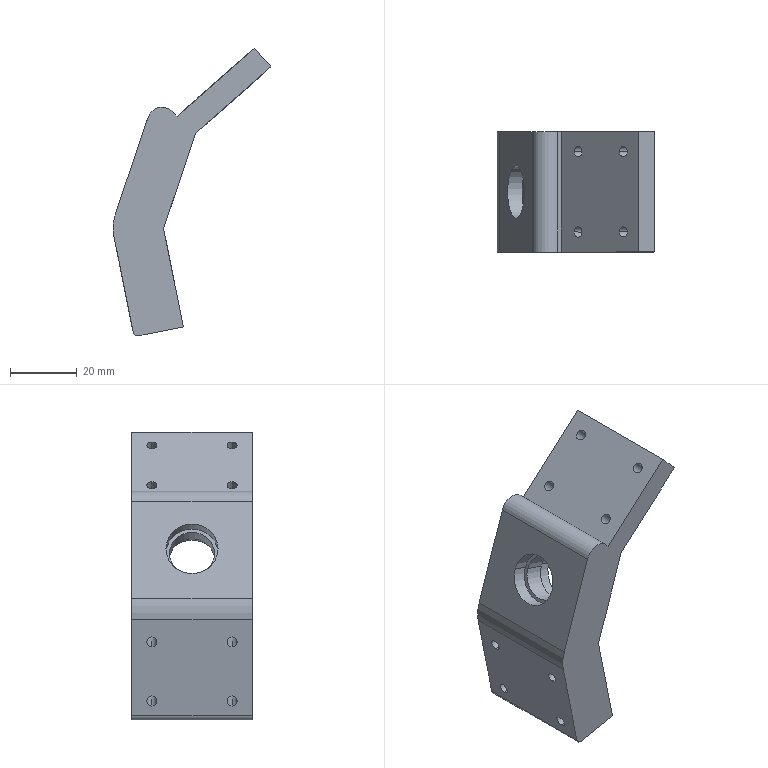Part | STEP file | 2026.6.15-Main Assembly图.sldasm-Part-275 | 1 solid | 38 faces | box 47.222 x 36 x 85.968 mm | volume 40942 mm3 | cylinder 25 | plane 13 | commonest cylinder face diameters 3.06 x16 15.6 x4 13.5 x2 3 x1 9 x1 24 x1
STEP:
#1=CARTESIAN_POINT('',(-1656.869,1431.014,3245.304));
#2=VERTEX_POINT('',#1);
#3=CARTESIAN_POINT('',(-1662.554,1431.014,3247.224));
#4=VERTEX_POINT('',#3);
#5=CARTESIAN_POINT('',(-1638.394,1431.014,3239.065));
#6=DIRECTION('',(-0.9474,0.,0.3199));
#7=VECTOR('',#6,1000.);
#8=LINE('',#5,#7);
#9=EDGE_CURVE('',#2,#4,#8,.T.);
#10=ORIENTED_EDGE('',*,*,#9,.F.);
#11=CARTESIAN_POINT('',(-1656.869,1417.514,3245.304));
#12=VERTEX_POINT('',#11);
#13=CARTESIAN_POINT('',(-1656.869,1424.264,3245.304));
#14=DIRECTION('',(-0.9474,0.,0.3199));
#15=DIRECTION('',(0.,-1.,0.));
#16=AXIS2_PLACEMENT_3D('',#13,#14,#15);
#17=CIRCLE('',#16,6.75);
#18=EDGE_CURVE('',#12,#2,#17,.T.);
#19=ORIENTED_EDGE('',*,*,#18,.F.);
#20=CARTESIAN_POINT('',(-1662.554,1417.514,3247.224));
#21=VERTEX_POINT('',#20);
#22=CARTESIAN_POINT('',(-1638.394,1417.514,3239.065));
#23=DIRECTION('',(-0.9474,0.,0.3199));
#24=VECTOR('',#23,1000.);
#25=LINE('',#22,#24);
#26=EDGE_CURVE('',#12,#21,#25,.T.);
#27=ORIENTED_EDGE('',*,*,#26,.T.);
#28=CARTESIAN_POINT('',(-1662.554,1424.264,3247.224));
#29=DIRECTION('',(0.9474,0.,-0.3199));
#30=DIRECTION('',(0.,-1.,0.));
#31=AXIS2_PLACEMENT_3D('',#28,#29,#30);
#32=CIRCLE('',#31,6.75);
#33=EDGE_CURVE('',#4,#21,#32,.T.);
#34=ORIENTED_EDGE('',*,*,#33,.F.);
#35=EDGE_LOOP('',(#10,#19,#27,#34));
#36=FACE_OUTER_BOUND('',#35,.T.);
#37=CARTESIAN_POINT('',(-1638.394,1424.264,3239.065));
#38=DIRECTION('',(-0.9474,0.,0.3199));
#39=DIRECTION('',(0.,1.,0.));
#40=AXIS2_PLACEMENT_3D('',#37,#38,#39);
#41=CYLINDRICAL_SURFACE('',#40,6.75);
#42=ADVANCED_FACE('',(#36),#41,.F.);
#43=CARTESIAN_POINT('',(-1662.554,1416.464,3247.224));
#44=VERTEX_POINT('',#43);
#45=CARTESIAN_POINT('',(-1662.554,1432.064,3247.224));
#46=VERTEX_POINT('',#45);
#47=CARTESIAN_POINT('',(-1662.554,1424.264,3247.224));
#48=DIRECTION('',(-0.9474,0.,0.3199));
#49=DIRECTION('',(0.,-1.,0.));
#50=AXIS2_PLACEMENT_3D('',#47,#48,#49);
#51=CIRCLE('',#50,7.8);
#52=EDGE_CURVE('',#44,#46,#51,.T.);
#53=ORIENTED_EDGE('',*,*,#52,.T.);
#54=CARTESIAN_POINT('',(-1662.554,1424.264,3247.224));
#55=DIRECTION('',(-0.9474,0.,0.3199));
#56=DIRECTION('',(0.,-1.,0.));
#57=AXIS2_PLACEMENT_3D('',#54,#55,#56);
#58=CIRCLE('',#57,7.8);
#59=EDGE_CURVE('',#46,#44,#58,.T.);
#60=ORIENTED_EDGE('',*,*,#59,.T.);
#61=EDGE_LOOP('',(#53,#60));
#62=FACE_OUTER_BOUND('',#61,.T.);
#63=CARTESIAN_POINT('',(-1662.554,1424.264,3247.224));
#64=DIRECTION('',(0.9474,0.,-0.3199));
#65=DIRECTION('',(0.,-1.,0.));
#66=AXIS2_PLACEMENT_3D('',#63,#64,#65);
#67=CIRCLE('',#66,6.75);
#68=EDGE_CURVE('',#21,#4,#67,.T.);
#69=ORIENTED_EDGE('',*,*,#68,.T.);
#70=ORIENTED_EDGE('',*,*,#33,.T.);
#71=EDGE_LOOP('',(#69,#70));
#72=FACE_BOUND('',#71,.T.);
#73=CARTESIAN_POINT('',(-1662.554,1424.264,3247.224));
#74=DIRECTION('',(-0.9474,0.,0.3199));
#75=DIRECTION('',(0.,1.,0.));
#76=AXIS2_PLACEMENT_3D('',#73,#74,#75);
#77=PLANE('',#76);
#78=ADVANCED_FACE('',(#62,#72),#77,.T.);
#79=CARTESIAN_POINT('',(-1656.869,1432.064,3245.304));
#80=VERTEX_POINT('',#79);
#81=CARTESIAN_POINT('',(-1656.869,1416.464,3245.304));
#82=VERTEX_POINT('',#81);
#83=CARTESIAN_POINT('',(-1656.869,1424.264,3245.304));
#84=DIRECTION('',(0.9474,0.,-0.3199));
#85=DIRECTION('',(0.,1.,0.));
#86=AXIS2_PLACEMENT_3D('',#83,#84,#85);
#87=CIRCLE('',#86,7.8);
#88=EDGE_CURVE('',#80,#82,#87,.T.);
#89=ORIENTED_EDGE('',*,*,#88,.T.);
#90=CARTESIAN_POINT('',(-1656.869,1424.264,3245.304));
#91=DIRECTION('',(0.9474,0.,-0.3199));
#92=DIRECTION('',(0.,1.,0.));
#93=AXIS2_PLACEMENT_3D('',#90,#91,#92);
#94=CIRCLE('',#93,7.8);
#95=EDGE_CURVE('',#82,#80,#94,.T.);
#96=ORIENTED_EDGE('',*,*,#95,.T.);
#97=EDGE_LOOP('',(#89,#96));
#98=FACE_OUTER_BOUND('',#97,.T.);
#99=ORIENTED_EDGE('',*,*,#18,.T.);
#100=CARTESIAN_POINT('',(-1656.869,1424.264,3245.304));
#101=DIRECTION('',(-0.9474,0.,0.3199));
#102=DIRECTION('',(0.,-1.,0.));
#103=AXIS2_PLACEMENT_3D('',#100,#101,#102);
#104=CIRCLE('',#103,6.75);
#105=EDGE_CURVE('',#2,#12,#104,.T.);
#106=ORIENTED_EDGE('',*,*,#105,.T.);
#107=EDGE_LOOP('',(#99,#106));
#108=FACE_BOUND('',#107,.T.);
#109=CARTESIAN_POINT('',(-1656.869,1424.264,3245.304));
#110=DIRECTION('',(0.9474,0.,-0.3199));
#111=DIRECTION('',(0.,-1.,0.));
#112=AXIS2_PLACEMENT_3D('',#109,#110,#111);
#113=PLANE('',#112);
#114=ADVANCED_FACE('',(#98,#108),#113,.T.);
#115=CARTESIAN_POINT('',(-1666.817,1432.064,3248.663));
#116=VERTEX_POINT('',#115);
#117=CARTESIAN_POINT('',(-1662.554,1432.064,3247.224));
#118=DIRECTION('',(-0.9474,0.,0.3199));
#119=VECTOR('',#118,1000.);
#120=LINE('',#117,#119);
#121=EDGE_CURVE('',#46,#116,#120,.T.);
#122=ORIENTED_EDGE('',*,*,#121,.F.);
#123=ORIENTED_EDGE('',*,*,#52,.F.);
#124=CARTESIAN_POINT('',(-1666.817,1416.464,3248.663));
#125=VERTEX_POINT('',#124);
#126=CARTESIAN_POINT('',(-1662.554,1416.464,3247.224));
#127=DIRECTION('',(-0.9474,0.,0.3199));
#128=VECTOR('',#127,1000.);
#129=LINE('',#126,#128);
#130=EDGE_CURVE('',#44,#125,#129,.T.);
#131=ORIENTED_EDGE('',*,*,#130,.T.);
#132=CARTESIAN_POINT('',(-1666.817,1424.264,3248.663));
#133=DIRECTION('',(-0.9474,0.,0.3199));
#134=DIRECTION('',(0.,-1.,0.));
#135=AXIS2_PLACEMENT_3D('',#132,#133,#134);
#136=CIRCLE('',#135,7.8);
#137=EDGE_CURVE('',#125,#116,#136,.T.);
#138=ORIENTED_EDGE('',*,*,#137,.T.);
#139=EDGE_LOOP('',(#122,#123,#131,#138));
#140=FACE_OUTER_BOUND('',#139,.T.);
#141=CARTESIAN_POINT('',(-1662.554,1424.264,3247.224));
#142=DIRECTION('',(-0.9474,0.,0.3199));
#143=DIRECTION('',(0.,1.,0.));
#144=AXIS2_PLACEMENT_3D('',#141,#142,#143);
#145=CYLINDRICAL_SURFACE('',#144,7.8);
#146=ADVANCED_FACE('',(#140),#145,.F.);
#147=CARTESIAN_POINT('',(-1655.924,1436.264,3222.27));
#148=VERTEX_POINT('',#147);
#149=CARTESIAN_POINT('',(-1670.631,1436.264,3219.32));
#150=VERTEX_POINT('',#149);
#151=CARTESIAN_POINT('',(-1655.924,1436.264,3222.27));
#152=DIRECTION('',(-0.9805,0.,-0.1966));
#153=VECTOR('',#152,1000.);
#154=LINE('',#151,#153);
#155=EDGE_CURVE('',#148,#150,#154,.T.);
#156=ORIENTED_EDGE('',*,*,#155,.T.);
#157=CARTESIAN_POINT('',(-1671.233,1436.264,3222.32));
#158=VERTEX_POINT('',#157);
#159=CARTESIAN_POINT('',(-1670.932,1436.264,3220.82));
#160=DIRECTION('',(-0.9805,0.,-0.1966));
#161=DIRECTION('',(-0.1966,0.,0.9805));
#162=AXIS2_PLACEMENT_3D('',#159,#160,#161);
#163=CIRCLE('',#162,1.53);
#164=EDGE_CURVE('',#150,#158,#163,.T.);
#165=ORIENTED_EDGE('',*,*,#164,.T.);
#166=CARTESIAN_POINT('',(-1656.526,1436.264,3225.27));
#167=VERTEX_POINT('',#166);
#168=CARTESIAN_POINT('',(-1656.526,1436.264,3225.27));
#169=DIRECTION('',(-0.9805,0.,-0.1966));
#170=VECTOR('',#169,1000.);
#171=LINE('',#168,#170);
#172=EDGE_CURVE('',#167,#158,#171,.T.);
#173=ORIENTED_EDGE('',*,*,#172,.F.);
#174=CARTESIAN_POINT('',(-1656.225,1436.264,3223.77));
#175=DIRECTION('',(0.9805,0.,0.1966));
#176=DIRECTION('',(-0.1966,0.,0.9805));
#177=AXIS2_PLACEMENT_3D('',#174,#175,#176);
#178=CIRCLE('',#177,1.53);
#179=EDGE_CURVE('',#167,#148,#178,.T.);
#180=ORIENTED_EDGE('',*,*,#179,.T.);
#181=EDGE_LOOP('',(#156,#165,#173,#180));
#182=FACE_OUTER_BOUND('',#181,.T.);
#183=CARTESIAN_POINT('',(-1656.225,1436.264,3223.77));
#184=DIRECTION('',(0.9805,0.,0.1966));
#185=DIRECTION('',(0.1966,0.,-0.9805));
#186=AXIS2_PLACEMENT_3D('',#183,#184,#185);
#187=CYLINDRICAL_SURFACE('',#186,1.53);
#188=ADVANCED_FACE('',(#182),#187,.F.);
#189=CARTESIAN_POINT('',(-1652.385,1436.264,3204.621));
#190=VERTEX_POINT('',#189);
#191=CARTESIAN_POINT('',(-1667.092,1436.264,3201.671));
#192=VERTEX_POINT('',#191);
#193=CARTESIAN_POINT('',(-1652.385,1436.264,3204.621));
#194=DIRECTION('',(-0.9805,0.,-0.1966));
#195=VECTOR('',#194,1000.);
#196=LINE('',#193,#195);
#197=EDGE_CURVE('',#190,#192,#196,.T.);
#198=ORIENTED_EDGE('',*,*,#197,.T.);
#199=CARTESIAN_POINT('',(-1667.694,1436.264,3204.672));
#200=VERTEX_POINT('',#199);
#201=CARTESIAN_POINT('',(-1667.393,1436.264,3203.172));
#202=DIRECTION('',(-0.9805,0.,-0.1966));
#203=DIRECTION('',(-0.1966,0.,0.9805));
#204=AXIS2_PLACEMENT_3D('',#201,#202,#203);
#205=CIRCLE('',#204,1.53);
#206=EDGE_CURVE('',#192,#200,#205,.T.);
#207=ORIENTED_EDGE('',*,*,#206,.T.);
#208=CARTESIAN_POINT('',(-1652.986,1436.264,3207.621));
#209=VERTEX_POINT('',#208);
#210=CARTESIAN_POINT('',(-1652.986,1436.264,3207.621));
#211=DIRECTION('',(-0.9805,0.,-0.1966));
#212=VECTOR('',#211,1000.);
#213=LINE('',#210,#212);
#214=EDGE_CURVE('',#209,#200,#213,.T.);
#215=ORIENTED_EDGE('',*,*,#214,.F.);
#216=CARTESIAN_POINT('',(-1652.686,1436.264,3206.121));
#217=DIRECTION('',(0.9805,0.,0.1966));
#218=DIRECTION('',(-0.1966,0.,0.9805));
#219=AXIS2_PLACEMENT_3D('',#216,#217,#218);
#220=CIRCLE('',#219,1.53);
#221=EDGE_CURVE('',#209,#190,#220,.T.);
#222=ORIENTED_EDGE('',*,*,#221,.T.);
#223=EDGE_LOOP('',(#198,#207,#215,#222));
#224=FACE_OUTER_BOUND('',#223,.T.);
#225=CARTESIAN_POINT('',(-1652.686,1436.264,3206.121));
#226=DIRECTION('',(0.9805,0.,0.1966));
#227=DIRECTION('',(0.1966,0.,-0.9805));
#228=AXIS2_PLACEMENT_3D('',#225,#226,#227);
#229=CYLINDRICAL_SURFACE('',#228,1.53);
#230=ADVANCED_FACE('',(#224),#229,.F.);
#231=CARTESIAN_POINT('',(-1655.924,1412.264,3222.27));
#232=VERTEX_POINT('',#231);
#233=CARTESIAN_POINT('',(-1670.631,1412.264,3219.32));
#234=VERTEX_POINT('',#233);
#235=CARTESIAN_POINT('',(-1655.924,1412.264,3222.27));
#236=DIRECTION('',(-0.9805,0.,-0.1966));
#237=VECTOR('',#236,1000.);
#238=LINE('',#235,#237);
#239=EDGE_CURVE('',#232,#234,#238,.T.);
#240=ORIENTED_EDGE('',*,*,#239,.T.);
#241=CARTESIAN_POINT('',(-1671.233,1412.264,3222.32));
#242=VERTEX_POINT('',#241);
#243=CARTESIAN_POINT('',(-1670.932,1412.264,3220.82));
#244=DIRECTION('',(-0.9805,0.,-0.1966));
#245=DIRECTION('',(-0.1966,0.,0.9805));
#246=AXIS2_PLACEMENT_3D('',#243,#244,#245);
#247=CIRCLE('',#246,1.53);
#248=EDGE_CURVE('',#234,#242,#247,.T.);
#249=ORIENTED_EDGE('',*,*,#248,.T.);
#250=CARTESIAN_POINT('',(-1656.526,1412.264,3225.27));
#251=VERTEX_POINT('',#250);
#252=CARTESIAN_POINT('',(-1656.526,1412.264,3225.27));
#253=DIRECTION('',(-0.9805,0.,-0.1966));
#254=VECTOR('',#253,1000.);
#255=LINE('',#252,#254);
#256=EDGE_CURVE('',#251,#242,#255,.T.);
#257=ORIENTED_EDGE('',*,*,#256,.F.);
#258=CARTESIAN_POINT('',(-1656.225,1412.264,3223.77));
#259=DIRECTION('',(0.9805,0.,0.1966));
#260=DIRECTION('',(-0.1966,0.,0.9805));
#261=AXIS2_PLACEMENT_3D('',#258,#259,#260);
#262=CIRCLE('',#261,1.53);
#263=EDGE_CURVE('',#251,#232,#262,.T.);
#264=ORIENTED_EDGE('',*,*,#263,.T.);
#265=EDGE_LOOP('',(#240,#249,#257,#264));
#266=FACE_OUTER_BOUND('',#265,.T.);
#267=CARTESIAN_POINT('',(-1656.225,1412.264,3223.77));
#268=DIRECTION('',(0.9805,0.,0.1966));
#269=DIRECTION('',(0.1966,0.,-0.9805));
#270=AXIS2_PLACEMENT_3D('',#267,#268,#269);
#271=CYLINDRICAL_SURFACE('',#270,1.53);
#272=ADVANCED_FACE('',(#266),#271,.F.);
#273=CARTESIAN_POINT('',(-1652.385,1412.264,3204.621));
#274=VERTEX_POINT('',#273);
#275=CARTESIAN_POINT('',(-1667.092,1412.264,3201.671));
#276=VERTEX_POINT('',#275);
#277=CARTESIAN_POINT('',(-1652.385,1412.264,3204.621));
#278=DIRECTION('',(-0.9805,0.,-0.1966));
#279=VECTOR('',#278,1000.);
#280=LINE('',#277,#279);
#281=EDGE_CURVE('',#274,#276,#280,.T.);
#282=ORIENTED_EDGE('',*,*,#281,.T.);
#283=CARTESIAN_POINT('',(-1667.694,1412.264,3204.672));
#284=VERTEX_POINT('',#283);
#285=CARTESIAN_POINT('',(-1667.393,1412.264,3203.172));
#286=DIRECTION('',(-0.9805,0.,-0.1966));
#287=DIRECTION('',(-0.1966,0.,0.9805));
#288=AXIS2_PLACEMENT_3D('',#285,#286,#287);
#289=CIRCLE('',#288,1.53);
#290=EDGE_CURVE('',#276,#284,#289,.T.);
#291=ORIENTED_EDGE('',*,*,#290,.T.);
#292=CARTESIAN_POINT('',(-1652.986,1412.264,3207.621));
#293=VERTEX_POINT('',#292);
#294=CARTESIAN_POINT('',(-1652.986,1412.264,3207.621));
#295=DIRECTION('',(-0.9805,0.,-0.1966));
#296=VECTOR('',#295,1000.);
#297=LINE('',#294,#296);
#298=EDGE_CURVE('',#293,#284,#297,.T.);
#299=ORIENTED_EDGE('',*,*,#298,.F.);
#300=CARTESIAN_POINT('',(-1652.686,1412.264,3206.121));
#301=DIRECTION('',(0.9805,0.,0.1966));
#302=DIRECTION('',(-0.1966,0.,0.9805));
#303=AXIS2_PLACEMENT_3D('',#300,#301,#302);
#304=CIRCLE('',#303,1.53);
#305=EDGE_CURVE('',#293,#274,#304,.T.);
#306=ORIENTED_EDGE('',*,*,#305,.T.);
#307=EDGE_LOOP('',(#282,#291,#299,#306));
#308=FACE_OUTER_BOUND('',#307,.T.);
#309=CARTESIAN_POINT('',(-1652.686,1412.264,3206.121));
#310=DIRECTION('',(0.9805,0.,0.1966));
#311=DIRECTION('',(0.1966,0.,-0.9805));
#312=AXIS2_PLACEMENT_3D('',#309,#310,#311);
#313=CYLINDRICAL_SURFACE('',#312,1.53);
#314=ADVANCED_FACE('',(#308),#313,.F.);
#315=CARTESIAN_POINT('',(-1652.606,1416.464,3243.864));
#316=VERTEX_POINT('',#315);
#317=CARTESIAN_POINT('',(-1656.869,1416.464,3245.304));
#318=DIRECTION('',(-0.9474,0.,0.3199));
#319=VECTOR('',#318,1000.);
#320=LINE('',#317,#319);
#321=EDGE_CURVE('',#316,#82,#320,.T.);
#322=ORIENTED_EDGE('',*,*,#321,.T.);
#323=ORIENTED_EDGE('',*,*,#88,.F.);
#324=CARTESIAN_POINT('',(-1652.606,1432.064,3243.864));
#325=VERTEX_POINT('',#324);
#326=CARTESIAN_POINT('',(-1656.869,1432.064,3245.304));
#327=DIRECTION('',(-0.9474,0.,0.3199));
#328=VECTOR('',#327,1000.);
#329=LINE('',#326,#328);
#330=EDGE_CURVE('',#325,#80,#329,.T.);
#331=ORIENTED_EDGE('',*,*,#330,.F.);
#332=CARTESIAN_POINT('',(-1652.606,1424.264,3243.864));
#333=DIRECTION('',(0.9474,0.,-0.3199));
#334=DIRECTION('',(0.,1.,0.));
#335=AXIS2_PLACEMENT_3D('',#332,#333,#334);
#336=CIRCLE('',#335,7.8);
#337=EDGE_CURVE('',#325,#316,#336,.T.);
#338=ORIENTED_EDGE('',*,*,#337,.T.);
#339=EDGE_LOOP('',(#322,#323,#331,#338));
#340=FACE_OUTER_BOUND('',#339,.T.);
#341=CARTESIAN_POINT('',(-1656.869,1424.264,3245.304));
#342=DIRECTION('',(0.9474,0.,-0.3199));
#343=DIRECTION('',(0.,-1.,0.));
#344=AXIS2_PLACEMENT_3D('',#341,#342,#343);
#345=CYLINDRICAL_SURFACE('',#344,7.8);
#346=ADVANCED_FACE('',(#340),#345,.F.);
#347=CARTESIAN_POINT('',(-1644.451,1412.264,3261.028));
#348=VERTEX_POINT('',#347);
#349=CARTESIAN_POINT('',(-1649.405,1412.264,3266.659));
#350=VERTEX_POINT('',#349);
#351=CARTESIAN_POINT('',(-1644.451,1412.264,3261.028));
#352=DIRECTION('',(-0.6605,0.,0.7508));
#353=VECTOR('',#352,1000.);
#354=LINE('',#351,#353);
#355=EDGE_CURVE('',#348,#350,#354,.T.);
#356=ORIENTED_EDGE('',*,*,#355,.T.);
#357=CARTESIAN_POINT('',(-1647.107,1412.264,3268.68));
#358=VERTEX_POINT('',#357);
#359=CARTESIAN_POINT('',(-1648.256,1412.264,3267.67));
#360=DIRECTION('',(-0.6605,0.,0.7508));
#361=DIRECTION('',(0.7508,0.,0.6605));
#362=AXIS2_PLACEMENT_3D('',#359,#360,#361);
#363=CIRCLE('',#362,1.53);
#364=EDGE_CURVE('',#350,#358,#363,.T.);
#365=ORIENTED_EDGE('',*,*,#364,.T.);
#366=CARTESIAN_POINT('',(-1642.153,1412.264,3263.049));
#367=VERTEX_POINT('',#366);
#368=CARTESIAN_POINT('',(-1642.153,1412.264,3263.049));
#369=DIRECTION('',(-0.6605,0.,0.7508));
#370=VECTOR('',#369,1000.);
#371=LINE('',#368,#370);
#372=EDGE_CURVE('',#367,#358,#371,.T.);
#373=ORIENTED_EDGE('',*,*,#372,.F.);
#374=CARTESIAN_POINT('',(-1643.302,1412.264,3262.039));
#375=DIRECTION('',(0.6605,0.,-0.7508));
#376=DIRECTION('',(0.7508,0.,0.6605));
#377=AXIS2_PLACEMENT_3D('',#374,#375,#376);
#378=CIRCLE('',#377,1.53);
#379=EDGE_CURVE('',#367,#348,#378,.T.);
#380=ORIENTED_EDGE('',*,*,#379,.T.);
#381=EDGE_LOOP('',(#356,#365,#373,#380));
#382=FACE_OUTER_BOUND('',#381,.T.);
#383=CARTESIAN_POINT('',(-1643.302,1412.264,3262.039));
#384=DIRECTION('',(0.6605,0.,-0.7508));
#385=DIRECTION('',(-0.7508,0.,-0.6605));
#386=AXIS2_PLACEMENT_3D('',#383,#384,#385);
#387=CYLINDRICAL_SURFACE('',#386,1.53);
#388=ADVANCED_FACE('',(#382),#387,.F.);
#389=CARTESIAN_POINT('',(-1644.451,1436.264,3261.028));
#390=VERTEX_POINT('',#389);
#391=CARTESIAN_POINT('',(-1649.405,1436.264,3266.659));
#392=VERTEX_POINT('',#391);
#393=CARTESIAN_POINT('',(-1644.451,1436.264,3261.028));
#394=DIRECTION('',(-0.6605,0.,0.7508));
#395=VECTOR('',#394,1000.);
#396=LINE('',#393,#395);
#397=EDGE_CURVE('',#390,#392,#396,.T.);
#398=ORIENTED_EDGE('',*,*,#397,.T.);
#399=CARTESIAN_POINT('',(-1647.107,1436.264,3268.68));
#400=VERTEX_POINT('',#399);
#401=CARTESIAN_POINT('',(-1648.256,1436.264,3267.67));
#402=DIRECTION('',(-0.6605,0.,0.7508));
#403=DIRECTION('',(0.7508,0.,0.6605));
#404=AXIS2_PLACEMENT_3D('',#401,#402,#403);
#405=CIRCLE('',#404,1.53);
#406=EDGE_CURVE('',#392,#400,#405,.T.);
#407=ORIENTED_EDGE('',*,*,#406,.T.);
#408=CARTESIAN_POINT('',(-1642.153,1436.264,3263.049));
#409=VERTEX_POINT('',#408);
#410=CARTESIAN_POINT('',(-1642.153,1436.264,3263.049));
#411=DIRECTION('',(-0.6605,0.,0.7508));
#412=VECTOR('',#411,1000.);
#413=LINE('',#410,#412);
#414=EDGE_CURVE('',#409,#400,#413,.T.);
#415=ORIENTED_EDGE('',*,*,#414,.F.);
#416=CARTESIAN_POINT('',(-1643.302,1436.264,3262.039));
#417=DIRECTION('',(0.6605,0.,-0.7508));
#418=DIRECTION('',(0.7508,0.,0.6605));
#419=AXIS2_PLACEMENT_3D('',#416,#417,#418);
#420=CIRCLE('',#419,1.53);
#421=EDGE_CURVE('',#409,#390,#420,.T.);
#422=ORIENTED_EDGE('',*,*,#421,.T.);
#423=EDGE_LOOP('',(#398,#407,#415,#422));
#424=FACE_OUTER_BOUND('',#423,.T.);
#425=CARTESIAN_POINT('',(-1643.302,1436.264,3262.039));
#426=DIRECTION('',(0.6605,0.,-0.7508));
#427=DIRECTION('',(-0.7508,0.,-0.6605));
#428=AXIS2_PLACEMENT_3D('',#425,#426,#427);
#429=CYLINDRICAL_SURFACE('',#428,1.53);
#430=ADVANCED_FACE('',(#424),#429,.F.);
#431=CARTESIAN_POINT('',(-1654.396,1442.264,3264.349));
#432=VERTEX_POINT('',#431);
#433=CARTESIAN_POINT('',(-1662.038,1442.264,3262.816));
#434=VERTEX_POINT('',#433);
#435=CARTESIAN_POINT('',(-1657.775,1442.264,3261.376));
#436=DIRECTION('',(0.,-1.,0.));
#437=DIRECTION('',(0.9474,0.,-0.3199));
#438=AXIS2_PLACEMENT_3D('',#435,#436,#437);
#439=CIRCLE('',#438,4.5);
#440=EDGE_CURVE('',#432,#434,#439,.T.);
#441=ORIENTED_EDGE('',*,*,#440,.F.);
#442=CARTESIAN_POINT('',(-1653.364,1442.264,3263.176));
#443=VERTEX_POINT('',#442);
#444=CARTESIAN_POINT('',(-1658.318,1442.264,3268.807));
#445=DIRECTION('',(0.6605,0.,-0.7508));
#446=VECTOR('',#445,1000.);
#447=LINE('',#444,#446);
#448=EDGE_CURVE('',#432,#443,#447,.T.);
#449=ORIENTED_EDGE('',*,*,#448,.T.);
#450=CARTESIAN_POINT('',(-1630.237,1442.264,3283.523));
#451=VERTEX_POINT('',#450);
#452=CARTESIAN_POINT('',(-1653.364,1442.264,3263.176));
#453=DIRECTION('',(0.7508,0.,0.6605));
#454=VECTOR('',#453,1000.);
#455=LINE('',#452,#454);
#456=EDGE_CURVE('',#443,#451,#455,.T.);
#457=ORIENTED_EDGE('',*,*,#456,.T.);
#458=CARTESIAN_POINT('',(-1625.283,1442.264,3277.892));
#459=VERTEX_POINT('',#458);
#460=CARTESIAN_POINT('',(-1625.283,1442.264,3277.892));
#461=DIRECTION('',(0.6605,0.,-0.7508));
#462=VECTOR('',#461,1000.);
#463=LINE('',#460,#462);
#464=EDGE_CURVE('',#451,#459,#463,.T.);
#465=ORIENTED_EDGE('',*,*,#464,.T.);
#466=CARTESIAN_POINT('',(-1647.807,1442.264,3258.076));
#467=VERTEX_POINT('',#466);
#468=CARTESIAN_POINT('',(-1647.807,1442.264,3258.076));
#469=DIRECTION('',(-0.7508,0.,-0.6605));
#470=VECTOR('',#469,1000.);
#471=LINE('',#468,#470);
#472=EDGE_CURVE('',#459,#467,#471,.T.);
#473=ORIENTED_EDGE('',*,*,#472,.T.);
#474=CARTESIAN_POINT('',(-1657.405,1442.264,3229.653));
#475=VERTEX_POINT('',#474);
#476=CARTESIAN_POINT('',(-1657.405,1442.264,3229.653));
#477=DIRECTION('',(-0.3199,0.,-0.9474));
#478=VECTOR('',#477,1000.);
#479=LINE('',#476,#478);
#480=EDGE_CURVE('',#467,#475,#479,.T.);
#481=ORIENTED_EDGE('',*,*,#480,.T.);
#482=CARTESIAN_POINT('',(-1651.506,1442.264,3200.238));
#483=VERTEX_POINT('',#482);
#484=CARTESIAN_POINT('',(-1657.405,1442.264,3229.653));
#485=DIRECTION('',(0.1966,0.,-0.9805));
#486=VECTOR('',#485,1000.);
#487=LINE('',#484,#486);
#488=EDGE_CURVE('',#475,#483,#487,.T.);
#489=ORIENTED_EDGE('',*,*,#488,.T.);
#490=CARTESIAN_POINT('',(-1664.742,1442.264,3197.584));
#491=VERTEX_POINT('',#490);
#492=CARTESIAN_POINT('',(-1651.506,1442.264,3200.238));
#493=DIRECTION('',(-0.9805,0.,-0.1966));
#494=VECTOR('',#493,1000.);
#495=LINE('',#492,#494);
#496=EDGE_CURVE('',#483,#491,#495,.T.);
#497=ORIENTED_EDGE('',*,*,#496,.T.);
#498=CARTESIAN_POINT('',(-1666.508,1442.264,3198.759));
#499=VERTEX_POINT('',#498);
#500=CARTESIAN_POINT('',(-1665.037,1442.264,3199.054));
#501=DIRECTION('',(0.,-1.,0.));
#502=DIRECTION('',(-0.9474,0.,0.3199));
#503=AXIS2_PLACEMENT_3D('',#500,#501,#502);
#504=CIRCLE('',#503,1.5);
#505=EDGE_CURVE('',#499,#491,#504,.T.);
#506=ORIENTED_EDGE('',*,*,#505,.F.);
#507=CARTESIAN_POINT('',(-1672.27,1442.264,3227.491));
#508=VERTEX_POINT('',#507);
#509=CARTESIAN_POINT('',(-1672.902,1442.264,3230.644));
#510=DIRECTION('',(-0.1966,0.,0.9805));
#511=VECTOR('',#510,1000.);
#512=LINE('',#509,#511);
#513=EDGE_CURVE('',#499,#508,#512,.T.);
#514=ORIENTED_EDGE('',*,*,#513,.T.);
#515=CARTESIAN_POINT('',(-1671.874,1442.264,3233.69));
#516=VERTEX_POINT('',#515);
#517=CARTESIAN_POINT('',(-1660.504,1442.264,3229.851));
#518=DIRECTION('',(0.,-1.,0.));
#519=DIRECTION('',(-0.9474,0.,0.3199));
#520=AXIS2_PLACEMENT_3D('',#517,#518,#519);
#521=CIRCLE('',#520,12.);
#522=EDGE_CURVE('',#516,#508,#521,.T.);
#523=ORIENTED_EDGE('',*,*,#522,.F.);
#524=CARTESIAN_POINT('',(-1672.902,1442.264,3230.644));
#525=DIRECTION('',(0.3199,0.,0.9474));
#526=VECTOR('',#525,1000.);
#527=LINE('',#524,#526);
#528=EDGE_CURVE('',#516,#434,#527,.T.);
#529=ORIENTED_EDGE('',*,*,#528,.T.);
#530=EDGE_LOOP('',(#441,#449,#457,#465,#473,#481,#489,#497,#506,#514,#523,#529));
#531=FACE_OUTER_BOUND('',#530,.T.);
#532=CARTESIAN_POINT('',(-1610.443,1442.264,3229.626));
#533=DIRECTION('',(0.,-1.,0.));
#534=DIRECTION('',(0.,0.,-1.));
#535=AXIS2_PLACEMENT_3D('',#532,#533,#534);
#536=PLANE('',#535);
#537=ADVANCED_FACE('',(#531),#536,.F.);
#538=CARTESIAN_POINT('',(-1630.936,1436.264,3272.918));
#539=VERTEX_POINT('',#538);
#540=CARTESIAN_POINT('',(-1635.89,1436.264,3278.549));
#541=VERTEX_POINT('',#540);
#542=CARTESIAN_POINT('',(-1630.936,1436.264,3272.918));
#543=DIRECTION('',(-0.6605,0.,0.7508));
#544=VECTOR('',#543,1000.);
#545=LINE('',#542,#544);
#546=EDGE_CURVE('',#539,#541,#545,.T.);
#547=ORIENTED_EDGE('',*,*,#546,.T.);
#548=CARTESIAN_POINT('',(-1633.593,1436.264,3280.57));
#549=VERTEX_POINT('',#548);
#550=CARTESIAN_POINT('',(-1634.741,1436.264,3279.559));
#551=DIRECTION('',(-0.6605,0.,0.7508));
#552=DIRECTION('',(0.7508,0.,0.6605));
#553=AXIS2_PLACEMENT_3D('',#550,#551,#552);
#554=CIRCLE('',#553,1.53);
#555=EDGE_CURVE('',#541,#549,#554,.T.);
#556=ORIENTED_EDGE('',*,*,#555,.T.);
#557=CARTESIAN_POINT('',(-1628.639,1436.264,3274.939));
#558=VERTEX_POINT('',#557);
#559=CARTESIAN_POINT('',(-1628.639,1436.264,3274.939));
#560=DIRECTION('',(-0.6605,0.,0.7508));
#561=VECTOR('',#560,1000.);
#562=LINE('',#559,#561);
#563=EDGE_CURVE('',#558,#549,#562,.T.);
#564=ORIENTED_EDGE('',*,*,#563,.F.);
#565=CARTESIAN_POINT('',(-1629.788,1436.264,3273.928));
#566=DIRECTION('',(0.6605,0.,-0.7508));
#567=DIRECTION('',(0.7508,0.,0.6605));
#568=AXIS2_PLACEMENT_3D('',#565,#566,#567);
#569=CIRCLE('',#568,1.53);
#570=EDGE_CURVE('',#558,#539,#569,.T.);
#571=ORIENTED_EDGE('',*,*,#570,.T.);
#572=EDGE_LOOP('',(#547,#556,#564,#571));
#573=FACE_OUTER_BOUND('',#572,.T.);
#574=CARTESIAN_POINT('',(-1629.788,1436.264,3273.928));
#575=DIRECTION('',(0.6605,0.,-0.7508));
#576=DIRECTION('',(-0.7508,0.,-0.6605));
#577=AXIS2_PLACEMENT_3D('',#574,#575,#576);
#578=CYLINDRICAL_SURFACE('',#577,1.53);
#579=ADVANCED_FACE('',(#573),#578,.F.);
#580=CARTESIAN_POINT('',(-1630.936,1412.264,3272.918));
#581=VERTEX_POINT('',#580);
#582=CARTESIAN_POINT('',(-1635.89,1412.264,3278.549));
#583=VERTEX_POINT('',#582);
#584=CARTESIAN_POINT('',(-1630.936,1412.264,3272.918));
#585=DIRECTION('',(-0.6605,0.,0.7508));
#586=VECTOR('',#585,1000.);
#587=LINE('',#584,#586);
#588=EDGE_CURVE('',#581,#583,#587,.T.);
#589=ORIENTED_EDGE('',*,*,#588,.T.);
#590=CARTESIAN_POINT('',(-1633.593,1412.264,3280.57));
#591=VERTEX_POINT('',#590);
#592=CARTESIAN_POINT('',(-1634.741,1412.264,3279.559));
#593=DIRECTION('',(-0.6605,0.,0.7508));
#594=DIRECTION('',(0.7508,0.,0.6605));
#595=AXIS2_PLACEMENT_3D('',#592,#593,#594);
#596=CIRCLE('',#595,1.53);
#597=EDGE_CURVE('',#583,#591,#596,.T.);
#598=ORIENTED_EDGE('',*,*,#597,.T.);
#599=CARTESIAN_POINT('',(-1628.639,1412.264,3274.939));
#600=VERTEX_POINT('',#599);
#601=CARTESIAN_POINT('',(-1628.639,1412.264,3274.939));
#602=DIRECTION('',(-0.6605,0.,0.7508));
#603=VECTOR('',#602,1000.);
#604=LINE('',#601,#603);
#605=EDGE_CURVE('',#600,#591,#604,.T.);
#606=ORIENTED_EDGE('',*,*,#605,.F.);
#607=CARTESIAN_POINT('',(-1629.788,1412.264,3273.928));
#608=DIRECTION('',(0.6605,0.,-0.7508));
#609=DIRECTION('',(0.7508,0.,0.6605));
#610=AXIS2_PLACEMENT_3D('',#607,#608,#609);
#611=CIRCLE('',#610,1.53);
#612=EDGE_CURVE('',#600,#581,#611,.T.);
#613=ORIENTED_EDGE('',*,*,#612,.T.);
#614=EDGE_LOOP('',(#589,#598,#606,#613));
#615=FACE_OUTER_BOUND('',#614,.T.);
#616=CARTESIAN_POINT('',(-1629.788,1412.264,3273.928));
#617=DIRECTION('',(0.6605,0.,-0.7508));
#618=DIRECTION('',(-0.7508,0.,-0.6605));
#619=AXIS2_PLACEMENT_3D('',#616,#617,#618);
#620=CYLINDRICAL_SURFACE('',#619,1.53);
#621=ADVANCED_FACE('',(#615),#620,.F.);
#622=CARTESIAN_POINT('',(-1654.396,1406.264,3264.349));
#623=VERTEX_POINT('',#622);
#624=CARTESIAN_POINT('',(-1654.396,1442.264,3264.349));
#625=DIRECTION('',(0.,1.,0.));
#626=VECTOR('',#625,1000.);
#627=LINE('',#624,#626);
#628=EDGE_CURVE('',#623,#432,#627,.T.);
#629=ORIENTED_EDGE('',*,*,#628,.F.);
#630=CARTESIAN_POINT('',(-1653.364,1406.264,3263.176));
#631=VERTEX_POINT('',#630);
#632=CARTESIAN_POINT('',(-1653.364,1406.264,3263.176));
#633=DIRECTION('',(-0.6605,0.,0.7508));
#634=VECTOR('',#633,1000.);
#635=LINE('',#632,#634);
#636=EDGE_CURVE('',#631,#623,#635,.T.);
#637=ORIENTED_EDGE('',*,*,#636,.F.);
#638=CARTESIAN_POINT('',(-1653.364,1442.264,3263.176));
#639=DIRECTION('',(0.,1.,0.));
#640=VECTOR('',#639,1000.);
#641=LINE('',#638,#640);
#642=EDGE_CURVE('',#631,#443,#641,.T.);
#643=ORIENTED_EDGE('',*,*,#642,.T.);
#644=ORIENTED_EDGE('',*,*,#448,.F.);
#645=EDGE_LOOP('',(#629,#637,#643,#644));
#646=FACE_OUTER_BOUND('',#645,.T.);
#647=CARTESIAN_POINT('',(-1658.318,1442.264,3268.807));
#648=DIRECTION('',(-0.7508,0.,-0.6605));
#649=DIRECTION('',(0.,1.,0.));
#650=AXIS2_PLACEMENT_3D('',#647,#648,#649);
#651=PLANE('',#650);
#652=ADVANCED_FACE('',(#646),#651,.F.);
#653=CARTESIAN_POINT('',(-1662.038,1406.264,3262.816));
#654=VERTEX_POINT('',#653);
#655=CARTESIAN_POINT('',(-1657.775,1406.264,3261.376));
#656=DIRECTION('',(0.,-1.,0.));
#657=DIRECTION('',(0.9474,0.,-0.3199));
#658=AXIS2_PLACEMENT_3D('',#655,#656,#657);
#659=CIRCLE('',#658,4.5);
#660=EDGE_CURVE('',#623,#654,#659,.T.);
#661=ORIENTED_EDGE('',*,*,#660,.F.);
#662=ORIENTED_EDGE('',*,*,#628,.T.);
#663=ORIENTED_EDGE('',*,*,#440,.T.);
#664=CARTESIAN_POINT('',(-1662.038,1406.264,3262.816));
#665=DIRECTION('',(0.,-1.,0.));
#666=VECTOR('',#665,1000.);
#667=LINE('',#664,#666);
#668=EDGE_CURVE('',#434,#654,#667,.T.);
#669=ORIENTED_EDGE('',*,*,#668,.T.);
#670=EDGE_LOOP('',(#661,#662,#663,#669));
#671=FACE_OUTER_BOUND('',#670,.T.);
#672=CARTESIAN_POINT('',(-1657.775,1442.264,3261.376));
#673=DIRECTION('',(0.,-1.,0.));
#674=DIRECTION('',(-0.9474,0.,0.3199));
#675=AXIS2_PLACEMENT_3D('',#672,#673,#674);
#676=CYLINDRICAL_SURFACE('',#675,4.5);
#677=ADVANCED_FACE('',(#671),#676,.T.);
#678=ORIENTED_EDGE('',*,*,#668,.F.);
#679=ORIENTED_EDGE('',*,*,#528,.F.);
#680=CARTESIAN_POINT('',(-1671.874,1406.264,3233.69));
#681=VERTEX_POINT('',#680);
#682=CARTESIAN_POINT('',(-1671.874,1406.264,3233.69));
#683=DIRECTION('',(0.,1.,0.));
#684=VECTOR('',#683,1000.);
#685=LINE('',#682,#684);
#686=EDGE_CURVE('',#681,#516,#685,.T.);
#687=ORIENTED_EDGE('',*,*,#686,.F.);
#688=CARTESIAN_POINT('',(-1666.817,1406.264,3248.663));
#689=DIRECTION('',(-0.3199,0.,-0.9474));
#690=VECTOR('',#689,1000.);
#691=LINE('',#688,#690);
#692=EDGE_CURVE('',#654,#681,#691,.T.);
#693=ORIENTED_EDGE('',*,*,#692,.F.);
#694=EDGE_LOOP('',(#678,#679,#687,#693));
#695=FACE_OUTER_BOUND('',#694,.T.);
#696=ORIENTED_EDGE('',*,*,#137,.F.);
#697=CARTESIAN_POINT('',(-1666.817,1424.264,3248.663));
#698=DIRECTION('',(-0.9474,0.,0.3199));
#699=DIRECTION('',(0.,-1.,0.));
#700=AXIS2_PLACEMENT_3D('',#697,#698,#699);
#701=CIRCLE('',#700,7.8);
#702=EDGE_CURVE('',#116,#125,#701,.T.);
#703=ORIENTED_EDGE('',*,*,#702,.F.);
#704=EDGE_LOOP('',(#696,#703));
#705=FACE_BOUND('',#704,.T.);
#706=CARTESIAN_POINT('',(-1672.902,1406.264,3230.644));
#707=DIRECTION('',(0.9474,0.,-0.3199));
#708=DIRECTION('',(0.,-1.,0.));
#709=AXIS2_PLACEMENT_3D('',#706,#707,#708);
#710=PLANE('',#709);
#711=ADVANCED_FACE('',(#695,#705),#710,.F.);
#712=ORIENTED_EDGE('',*,*,#522,.T.);
#713=CARTESIAN_POINT('',(-1672.27,1406.264,3227.491));
#714=VERTEX_POINT('',#713);
#715=CARTESIAN_POINT('',(-1672.27,1406.264,3227.491));
#716=DIRECTION('',(0.,-1.,0.));
#717=VECTOR('',#716,1000.);
#718=LINE('',#715,#717);
#719=EDGE_CURVE('',#508,#714,#718,.T.);
#720=ORIENTED_EDGE('',*,*,#719,.T.);
#721=CARTESIAN_POINT('',(-1660.504,1406.264,3229.851));
#722=DIRECTION('',(0.,-1.,0.));
#723=DIRECTION('',(-0.9474,0.,0.3199));
#724=AXIS2_PLACEMENT_3D('',#721,#722,#723);
#725=CIRCLE('',#724,12.);
#726=EDGE_CURVE('',#681,#714,#725,.T.);
#727=ORIENTED_EDGE('',*,*,#726,.F.);
#728=ORIENTED_EDGE('',*,*,#686,.T.);
#729=EDGE_LOOP('',(#712,#720,#727,#728));
#730=FACE_OUTER_BOUND('',#729,.T.);
#731=CARTESIAN_POINT('',(-1660.504,1406.264,3229.851));
#732=DIRECTION('',(0.,1.,0.));
#733=DIRECTION('',(0.9474,0.,-0.3199));
#734=AXIS2_PLACEMENT_3D('',#731,#732,#733);
#735=CYLINDRICAL_SURFACE('',#734,12.);
#736=ADVANCED_FACE('',(#730),#735,.T.);
#737=ORIENTED_EDGE('',*,*,#719,.F.);
#738=ORIENTED_EDGE('',*,*,#513,.F.);
#739=CARTESIAN_POINT('',(-1666.508,1406.264,3198.759));
#740=VERTEX_POINT('',#739);
#741=CARTESIAN_POINT('',(-1666.508,1406.264,3198.759));
#742=DIRECTION('',(0.,1.,0.));
#743=VECTOR('',#742,1000.);
#744=LINE('',#741,#743);
#745=EDGE_CURVE('',#740,#499,#744,.T.);
#746=ORIENTED_EDGE('',*,*,#745,.F.);
#747=CARTESIAN_POINT('',(-1672.27,1406.264,3227.491));
#748=DIRECTION('',(0.1966,0.,-0.9805));
#749=VECTOR('',#748,1000.);
#750=LINE('',#747,#749);
#751=EDGE_CURVE('',#714,#740,#750,.T.);
#752=ORIENTED_EDGE('',*,*,#751,.F.);
#753=EDGE_LOOP('',(#737,#738,#746,#752));
#754=FACE_OUTER_BOUND('',#753,.T.);
#755=CARTESIAN_POINT('',(-1670.932,1436.264,3220.82));
#756=DIRECTION('',(-0.9805,0.,-0.1966));
#757=DIRECTION('',(-0.1966,0.,0.9805));
#758=AXIS2_PLACEMENT_3D('',#755,#756,#757);
#759=CIRCLE('',#758,1.53);
#760=EDGE_CURVE('',#158,#150,#759,.T.);
#761=ORIENTED_EDGE('',*,*,#760,.F.);
#762=ORIENTED_EDGE('',*,*,#164,.F.);
#763=EDGE_LOOP('',(#761,#762));
#764=FACE_BOUND('',#763,.T.);
#765=CARTESIAN_POINT('',(-1667.393,1436.264,3203.172));
#766=DIRECTION('',(-0.9805,0.,-0.1966));
#767=DIRECTION('',(-0.1966,0.,0.9805));
#768=AXIS2_PLACEMENT_3D('',#765,#766,#767);
#769=CIRCLE('',#768,1.53);
#770=EDGE_CURVE('',#200,#192,#769,.T.);
#771=ORIENTED_EDGE('',*,*,#770,.F.);
#772=ORIENTED_EDGE('',*,*,#206,.F.);
#773=EDGE_LOOP('',(#771,#772));
#774=FACE_BOUND('',#773,.T.);
#775=CARTESIAN_POINT('',(-1670.932,1412.264,3220.82));
#776=DIRECTION('',(-0.9805,0.,-0.1966));
#777=DIRECTION('',(-0.1966,0.,0.9805));
#778=AXIS2_PLACEMENT_3D('',#775,#776,#777);
#779=CIRCLE('',#778,1.53);
#780=EDGE_CURVE('',#242,#234,#779,.T.);
#781=ORIENTED_EDGE('',*,*,#780,.F.);
#782=ORIENTED_EDGE('',*,*,#248,.F.);
#783=EDGE_LOOP('',(#781,#782));
#784=FACE_BOUND('',#783,.T.);
#785=CARTESIAN_POINT('',(-1667.393,1412.264,3203.172));
#786=DIRECTION('',(-0.9805,0.,-0.1966));
#787=DIRECTION('',(-0.1966,0.,0.9805));
#788=AXIS2_PLACEMENT_3D('',#785,#786,#787);
#789=CIRCLE('',#788,1.53);
#790=EDGE_CURVE('',#284,#276,#789,.T.);
#791=ORIENTED_EDGE('',*,*,#790,.F.);
#792=ORIENTED_EDGE('',*,*,#290,.F.);
#793=EDGE_LOOP('',(#791,#792));
#794=FACE_BOUND('',#793,.T.);
#795=CARTESIAN_POINT('',(-1672.902,1406.264,3230.644));
#796=DIRECTION('',(0.9805,0.,0.1966));
#797=DIRECTION('',(-0.1966,0.,0.9805));
#798=AXIS2_PLACEMENT_3D('',#795,#796,#797);
#799=PLANE('',#798);
#800=ADVANCED_FACE('',(#754,#764,#774,#784,#794),#799,.F.);
#801=ORIENTED_EDGE('',*,*,#505,.T.);
#802=CARTESIAN_POINT('',(-1664.742,1406.264,3197.584));
#803=VERTEX_POINT('',#802);
#804=CARTESIAN_POINT('',(-1664.742,1406.264,3197.584));
#805=DIRECTION('',(0.,-1.,0.));
#806=VECTOR('',#805,1000.);
#807=LINE('',#804,#806);
#808=EDGE_CURVE('',#491,#803,#807,.T.);
#809=ORIENTED_EDGE('',*,*,#808,.T.);
#810=CARTESIAN_POINT('',(-1665.037,1406.264,3199.054));
#811=DIRECTION('',(0.,-1.,0.));
#812=DIRECTION('',(-0.9474,0.,0.3199));
#813=AXIS2_PLACEMENT_3D('',#810,#811,#812);
#814=CIRCLE('',#813,1.5);
#815=EDGE_CURVE('',#740,#803,#814,.T.);
#816=ORIENTED_EDGE('',*,*,#815,.F.);
#817=ORIENTED_EDGE('',*,*,#745,.T.);
#818=EDGE_LOOP('',(#801,#809,#816,#817));
#819=FACE_OUTER_BOUND('',#818,.T.);
#820=CARTESIAN_POINT('',(-1665.037,1406.264,3199.054));
#821=DIRECTION('',(0.,1.,0.));
#822=DIRECTION('',(0.9474,0.,-0.3199));
#823=AXIS2_PLACEMENT_3D('',#820,#821,#822);
#824=CYLINDRICAL_SURFACE('',#823,1.5);
#825=ADVANCED_FACE('',(#819),#824,.T.);
#826=ORIENTED_EDGE('',*,*,#808,.F.);
#827=ORIENTED_EDGE('',*,*,#496,.F.);
#828=CARTESIAN_POINT('',(-1651.506,1406.264,3200.238));
#829=VERTEX_POINT('',#828);
#830=CARTESIAN_POINT('',(-1651.506,1406.264,3200.238));
#831=DIRECTION('',(0.,-1.,0.));
#832=VECTOR('',#831,1000.);
#833=LINE('',#830,#832);
#834=EDGE_CURVE('',#483,#829,#833,.T.);
#835=ORIENTED_EDGE('',*,*,#834,.T.);
#836=CARTESIAN_POINT('',(-1664.742,1406.264,3197.584));
#837=DIRECTION('',(0.9805,0.,0.1966));
#838=VECTOR('',#837,1000.);
#839=LINE('',#836,#838);
#840=EDGE_CURVE('',#803,#829,#839,.T.);
#841=ORIENTED_EDGE('',*,*,#840,.F.);
#842=EDGE_LOOP('',(#826,#827,#835,#841));
#843=FACE_OUTER_BOUND('',#842,.T.);
#844=CARTESIAN_POINT('',(-1651.506,1406.264,3200.238));
#845=DIRECTION('',(-0.1966,0.,0.9805));
#846=DIRECTION('',(0.,1.,0.));
#847=AXIS2_PLACEMENT_3D('',#844,#845,#846);
#848=PLANE('',#847);
#849=ADVANCED_FACE('',(#843),#848,.F.);
#850=CARTESIAN_POINT('',(-1657.405,1406.264,3229.653));
#851=VERTEX_POINT('',#850);
#852=CARTESIAN_POINT('',(-1657.405,1406.264,3229.653));
#853=DIRECTION('',(0.,-1.,0.));
#854=VECTOR('',#853,1000.);
#855=LINE('',#852,#854);
#856=EDGE_CURVE('',#475,#851,#855,.T.);
#857=ORIENTED_EDGE('',*,*,#856,.T.);
#858=CARTESIAN_POINT('',(-1651.506,1406.264,3200.238));
#859=DIRECTION('',(-0.1966,0.,0.9805));
#860=VECTOR('',#859,1000.);
#861=LINE('',#858,#860);
#862=EDGE_CURVE('',#829,#851,#861,.T.);
#863=ORIENTED_EDGE('',*,*,#862,.F.);
#864=ORIENTED_EDGE('',*,*,#834,.F.);
#865=ORIENTED_EDGE('',*,*,#488,.F.);
#866=EDGE_LOOP('',(#857,#863,#864,#865));
#867=FACE_OUTER_BOUND('',#866,.T.);
#868=ORIENTED_EDGE('',*,*,#179,.F.);
#869=CARTESIAN_POINT('',(-1656.225,1436.264,3223.77));
#870=DIRECTION('',(0.9805,0.,0.1966));
#871=DIRECTION('',(-0.1966,0.,0.9805));
#872=AXIS2_PLACEMENT_3D('',#869,#870,#871);
#873=CIRCLE('',#872,1.53);
#874=EDGE_CURVE('',#148,#167,#873,.T.);
#875=ORIENTED_EDGE('',*,*,#874,.F.);
#876=EDGE_LOOP('',(#868,#875));
#877=FACE_BOUND('',#876,.T.);
#878=ORIENTED_EDGE('',*,*,#221,.F.);
#879=CARTESIAN_POINT('',(-1652.686,1436.264,3206.121));
#880=DIRECTION('',(0.9805,0.,0.1966));
#881=DIRECTION('',(-0.1966,0.,0.9805));
#882=AXIS2_PLACEMENT_3D('',#879,#880,#881);
#883=CIRCLE('',#882,1.53);
#884=EDGE_CURVE('',#190,#209,#883,.T.);
#885=ORIENTED_EDGE('',*,*,#884,.F.);
#886=EDGE_LOOP('',(#878,#885));
#887=FACE_BOUND('',#886,.T.);
#888=ORIENTED_EDGE('',*,*,#263,.F.);
#889=CARTESIAN_POINT('',(-1656.225,1412.264,3223.77));
#890=DIRECTION('',(0.9805,0.,0.1966));
#891=DIRECTION('',(-0.1966,0.,0.9805));
#892=AXIS2_PLACEMENT_3D('',#889,#890,#891);
#893=CIRCLE('',#892,1.53);
#894=EDGE_CURVE('',#232,#251,#893,.T.);
#895=ORIENTED_EDGE('',*,*,#894,.F.);
#896=EDGE_LOOP('',(#888,#895));
#897=FACE_BOUND('',#896,.T.);
#898=ORIENTED_EDGE('',*,*,#305,.F.);
#899=CARTESIAN_POINT('',(-1652.686,1412.264,3206.121));
#900=DIRECTION('',(0.9805,0.,0.1966));
#901=DIRECTION('',(-0.1966,0.,0.9805));
#902=AXIS2_PLACEMENT_3D('',#899,#900,#901);
#903=CIRCLE('',#902,1.53);
#904=EDGE_CURVE('',#274,#293,#903,.T.);
#905=ORIENTED_EDGE('',*,*,#904,.F.);
#906=EDGE_LOOP('',(#898,#905));
#907=FACE_BOUND('',#906,.T.);
#908=CARTESIAN_POINT('',(-1657.405,1406.264,3229.653));
#909=DIRECTION('',(-0.9805,0.,-0.1966));
#910=DIRECTION('',(0.,1.,0.));
#911=AXIS2_PLACEMENT_3D('',#908,#909,#910);
#912=PLANE('',#911);
#913=ADVANCED_FACE('',(#867,#877,#887,#897,#907),#912,.F.);
#914=CARTESIAN_POINT('',(-1647.807,1406.264,3258.076));
#915=VERTEX_POINT('',#914);
#916=CARTESIAN_POINT('',(-1647.807,1406.264,3258.076));
#917=DIRECTION('',(0.,-1.,0.));
#918=VECTOR('',#917,1000.);
#919=LINE('',#916,#918);
#920=EDGE_CURVE('',#467,#915,#919,.T.);
#921=ORIENTED_EDGE('',*,*,#920,.T.);
#922=CARTESIAN_POINT('',(-1652.606,1406.264,3243.864));
#923=DIRECTION('',(0.3199,0.,0.9474));
#924=VECTOR('',#923,1000.);
#925=LINE('',#922,#924);
#926=EDGE_CURVE('',#851,#915,#925,.T.);
#927=ORIENTED_EDGE('',*,*,#926,.F.);
#928=ORIENTED_EDGE('',*,*,#856,.F.);
#929=ORIENTED_EDGE('',*,*,#480,.F.);
#930=EDGE_LOOP('',(#921,#927,#928,#929));
#931=FACE_OUTER_BOUND('',#930,.T.);
#932=ORIENTED_EDGE('',*,*,#337,.F.);
#933=CARTESIAN_POINT('',(-1652.606,1424.264,3243.864));
#934=DIRECTION('',(0.9474,0.,-0.3199));
#935=DIRECTION('',(0.,1.,0.));
#936=AXIS2_PLACEMENT_3D('',#933,#934,#935);
#937=CIRCLE('',#936,7.8);
#938=EDGE_CURVE('',#316,#325,#937,.T.);
#939=ORIENTED_EDGE('',*,*,#938,.F.);
#940=EDGE_LOOP('',(#932,#939));
#941=FACE_BOUND('',#940,.T.);
#942=CARTESIAN_POINT('',(-1657.405,1406.264,3229.653));
#943=DIRECTION('',(-0.9474,0.,0.3199));
#944=DIRECTION('',(0.,1.,0.));
#945=AXIS2_PLACEMENT_3D('',#942,#943,#944);
#946=PLANE('',#945);
#947=ADVANCED_FACE('',(#931,#941),#946,.F.);
#948=CARTESIAN_POINT('',(-1625.283,1406.264,3277.892));
#949=VERTEX_POINT('',#948);
#950=CARTESIAN_POINT('',(-1625.283,1406.264,3277.892));
#951=DIRECTION('',(0.,-1.,0.));
#952=VECTOR('',#951,1000.);
#953=LINE('',#950,#952);
#954=EDGE_CURVE('',#459,#949,#953,.T.);
#955=ORIENTED_EDGE('',*,*,#954,.T.);
#956=CARTESIAN_POINT('',(-1647.807,1406.264,3258.076));
#957=DIRECTION('',(0.7508,0.,0.6605));
#958=VECTOR('',#957,1000.);
#959=LINE('',#956,#958);
#960=EDGE_CURVE('',#915,#949,#959,.T.);
#961=ORIENTED_EDGE('',*,*,#960,.F.);
#962=ORIENTED_EDGE('',*,*,#920,.F.);
#963=ORIENTED_EDGE('',*,*,#472,.F.);
#964=EDGE_LOOP('',(#955,#961,#962,#963));
#965=FACE_OUTER_BOUND('',#964,.T.);
#966=ORIENTED_EDGE('',*,*,#421,.F.);
#967=CARTESIAN_POINT('',(-1643.302,1436.264,3262.039));
#968=DIRECTION('',(0.6605,0.,-0.7508));
#969=DIRECTION('',(0.7508,0.,0.6605));
#970=AXIS2_PLACEMENT_3D('',#967,#968,#969);
#971=CIRCLE('',#970,1.53);
#972=EDGE_CURVE('',#390,#409,#971,.T.);
#973=ORIENTED_EDGE('',*,*,#972,.F.);
#974=EDGE_LOOP('',(#966,#973));
#975=FACE_BOUND('',#974,.T.);
#976=ORIENTED_EDGE('',*,*,#570,.F.);
#977=CARTESIAN_POINT('',(-1629.788,1436.264,3273.928));
#978=DIRECTION('',(0.6605,0.,-0.7508));
#979=DIRECTION('',(0.7508,0.,0.6605));
#980=AXIS2_PLACEMENT_3D('',#977,#978,#979);
#981=CIRCLE('',#980,1.53);
#982=EDGE_CURVE('',#539,#558,#981,.T.);
#983=ORIENTED_EDGE('',*,*,#982,.F.);
#984=EDGE_LOOP('',(#976,#983));
#985=FACE_BOUND('',#984,.T.);
#986=ORIENTED_EDGE('',*,*,#379,.F.);
#987=CARTESIAN_POINT('',(-1643.302,1412.264,3262.039));
#988=DIRECTION('',(0.6605,0.,-0.7508));
#989=DIRECTION('',(0.7508,0.,0.6605));
#990=AXIS2_PLACEMENT_3D('',#987,#988,#989);
#991=CIRCLE('',#990,1.53);
#992=EDGE_CURVE('',#348,#367,#991,.T.);
#993=ORIENTED_EDGE('',*,*,#992,.F.);
#994=EDGE_LOOP('',(#986,#993));
#995=FACE_BOUND('',#994,.T.);
#996=ORIENTED_EDGE('',*,*,#612,.F.);
#997=CARTESIAN_POINT('',(-1629.788,1412.264,3273.928));
#998=DIRECTION('',(0.6605,0.,-0.7508));
#999=DIRECTION('',(0.7508,0.,0.6605));
#1000=AXIS2_PLACEMENT_3D('',#997,#998,#999);
#1001=CIRCLE('',#1000,1.53);
#1002=EDGE_CURVE('',#581,#600,#1001,.T.);
#1003=ORIENTED_EDGE('',*,*,#1002,.F.);
#1004=EDGE_LOOP('',(#996,#1003));
#1005=FACE_BOUND('',#1004,.T.);
#1006=CARTESIAN_POINT('',(-1647.807,1406.264,3258.076));
#1007=DIRECTION('',(-0.6605,0.,0.7508));
#1008=DIRECTION('',(0.,1.,0.));
#1009=AXIS2_PLACEMENT_3D('',#1006,#1007,#1008);
#1010=PLANE('',#1009);
#1011=ADVANCED_FACE('',(#965,#975,#985,#995,#1005),#1010,.F.);
#1012=CARTESIAN_POINT('',(-1630.237,1406.264,3283.523));
#1013=VERTEX_POINT('',#1012);
#1014=CARTESIAN_POINT('',(-1630.237,1442.264,3283.523));
#1015=DIRECTION('',(0.,-1.,0.));
#1016=VECTOR('',#1015,1000.);
#1017=LINE('',#1014,#1016);
#1018=EDGE_CURVE('',#451,#1013,#1017,.T.);
#1019=ORIENTED_EDGE('',*,*,#1018,.T.);
#1020=CARTESIAN_POINT('',(-1625.283,1406.264,3277.892));
#1021=DIRECTION('',(-0.6605,0.,0.7508));
#1022=VECTOR('',#1021,1000.);
#1023=LINE('',#1020,#1022);
#1024=EDGE_CURVE('',#949,#1013,#1023,.T.);
#1025=ORIENTED_EDGE('',*,*,#1024,.F.);
#1026=ORIENTED_EDGE('',*,*,#954,.F.);
#1027=ORIENTED_EDGE('',*,*,#464,.F.);
#1028=EDGE_LOOP('',(#1019,#1025,#1026,#1027));
#1029=FACE_OUTER_BOUND('',#1028,.T.);
#1030=CARTESIAN_POINT('',(-1625.283,1406.264,3277.892));
#1031=DIRECTION('',(-0.7508,0.,-0.6605));
#1032=DIRECTION('',(0.,1.,0.));
#1033=AXIS2_PLACEMENT_3D('',#1030,#1031,#1032);
#1034=PLANE('',#1033);
#1035=ADVANCED_FACE('',(#1029),#1034,.F.);
#1036=ORIENTED_EDGE('',*,*,#1018,.F.);
#1037=ORIENTED_EDGE('',*,*,#456,.F.);
#1038=ORIENTED_EDGE('',*,*,#642,.F.);
#1039=CARTESIAN_POINT('',(-1630.237,1406.264,3283.523));
#1040=DIRECTION('',(-0.7508,0.,-0.6605));
#1041=VECTOR('',#1040,1000.);
#1042=LINE('',#1039,#1041);
#1043=EDGE_CURVE('',#1013,#631,#1042,.T.);
#1044=ORIENTED_EDGE('',*,*,#1043,.F.);
#1045=EDGE_LOOP('',(#1036,#1037,#1038,#1044));
#1046=FACE_OUTER_BOUND('',#1045,.T.);
#1047=CARTESIAN_POINT('',(-1648.256,1412.264,3267.67));
#1048=DIRECTION('',(-0.6605,0.,0.7508));
#1049=DIRECTION('',(0.7508,0.,0.6605));
#1050=AXIS2_PLACEMENT_3D('',#1047,#1048,#1049);
#1051=CIRCLE('',#1050,1.53);
#1052=EDGE_CURVE('',#358,#350,#1051,.T.);
#1053=ORIENTED_EDGE('',*,*,#1052,.F.);
#1054=ORIENTED_EDGE('',*,*,#364,.F.);
#1055=EDGE_LOOP('',(#1053,#1054));
#1056=FACE_BOUND('',#1055,.T.);
#1057=CARTESIAN_POINT('',(-1648.256,1436.264,3267.67));
#1058=DIRECTION('',(-0.6605,0.,0.7508));
#1059=DIRECTION('',(0.7508,0.,0.6605));
#1060=AXIS2_PLACEMENT_3D('',#1057,#1058,#1059);
#1061=CIRCLE('',#1060,1.53);
#1062=EDGE_CURVE('',#400,#392,#1061,.T.);
#1063=ORIENTED_EDGE('',*,*,#1062,.F.);
#1064=ORIENTED_EDGE('',*,*,#406,.F.);
#1065=EDGE_LOOP('',(#1063,#1064));
#1066=FACE_BOUND('',#1065,.T.);
#1067=CARTESIAN_POINT('',(-1634.741,1436.264,3279.559));
#1068=DIRECTION('',(-0.6605,0.,0.7508));
#1069=DIRECTION('',(0.7508,0.,0.6605));
#1070=AXIS2_PLACEMENT_3D('',#1067,#1068,#1069);
#1071=CIRCLE('',#1070,1.53);
#1072=EDGE_CURVE('',#549,#541,#1071,.T.);
#1073=ORIENTED_EDGE('',*,*,#1072,.F.);
#1074=ORIENTED_EDGE('',*,*,#555,.F.);
#1075=EDGE_LOOP('',(#1073,#1074));
#1076=FACE_BOUND('',#1075,.T.);
#1077=CARTESIAN_POINT('',(-1634.741,1412.264,3279.559));
#1078=DIRECTION('',(-0.6605,0.,0.7508));
#1079=DIRECTION('',(0.7508,0.,0.6605));
#1080=AXIS2_PLACEMENT_3D('',#1077,#1078,#1079);
#1081=CIRCLE('',#1080,1.53);
#1082=EDGE_CURVE('',#591,#583,#1081,.T.);
#1083=ORIENTED_EDGE('',*,*,#1082,.F.);
#1084=ORIENTED_EDGE('',*,*,#597,.F.);
#1085=EDGE_LOOP('',(#1083,#1084));
#1086=FACE_BOUND('',#1085,.T.);
#1087=CARTESIAN_POINT('',(-1653.364,1442.264,3263.176));
#1088=DIRECTION('',(0.6605,0.,-0.7508));
#1089=DIRECTION('',(0.,-1.,0.));
#1090=AXIS2_PLACEMENT_3D('',#1087,#1088,#1089);
#1091=PLANE('',#1090);
#1092=ADVANCED_FACE('',(#1046,#1056,#1066,#1076,#1086),#1091,.F.);
#1093=ORIENTED_EDGE('',*,*,#1024,.T.);
#1094=ORIENTED_EDGE('',*,*,#1043,.T.);
#1095=ORIENTED_EDGE('',*,*,#636,.T.);
#1096=ORIENTED_EDGE('',*,*,#660,.T.);
#1097=ORIENTED_EDGE('',*,*,#692,.T.);
#1098=ORIENTED_EDGE('',*,*,#726,.T.);
#1099=ORIENTED_EDGE('',*,*,#751,.T.);
#1100=ORIENTED_EDGE('',*,*,#815,.T.);
#1101=ORIENTED_EDGE('',*,*,#840,.T.);
#1102=ORIENTED_EDGE('',*,*,#862,.T.);
#1103=ORIENTED_EDGE('',*,*,#926,.T.);
#1104=ORIENTED_EDGE('',*,*,#960,.T.);
#1105=EDGE_LOOP('',(#1093,#1094,#1095,#1096,#1097,#1098,#1099,#1100,#1101,#1102,#1103,#1104));
#1106=FACE_OUTER_BOUND('',#1105,.T.);
#1107=CARTESIAN_POINT('',(-1610.443,1406.264,3229.626));
#1108=DIRECTION('',(0.,-1.,0.));
#1109=DIRECTION('',(0.,0.,-1.));
#1110=AXIS2_PLACEMENT_3D('',#1107,#1108,#1109);
#1111=PLANE('',#1110);
#1112=ADVANCED_FACE('',(#1106),#1111,.T.);
#1113=ORIENTED_EDGE('',*,*,#105,.F.);
#1114=ORIENTED_EDGE('',*,*,#9,.T.);
#1115=ORIENTED_EDGE('',*,*,#68,.F.);
#1116=ORIENTED_EDGE('',*,*,#26,.F.);
#1117=EDGE_LOOP('',(#1113,#1114,#1115,#1116));
#1118=FACE_OUTER_BOUND('',#1117,.T.);
#1119=CARTESIAN_POINT('',(-1638.394,1424.264,3239.065));
#1120=DIRECTION('',(-0.9474,0.,0.3199));
#1121=DIRECTION('',(0.,1.,0.));
#1122=AXIS2_PLACEMENT_3D('',#1119,#1120,#1121);
#1123=CYLINDRICAL_SURFACE('',#1122,6.75);
#1124=ADVANCED_FACE('',(#1118),#1123,.F.);
#1125=ORIENTED_EDGE('',*,*,#59,.F.);
#1126=ORIENTED_EDGE('',*,*,#121,.T.);
#1127=ORIENTED_EDGE('',*,*,#702,.T.);
#1128=ORIENTED_EDGE('',*,*,#130,.F.);
#1129=EDGE_LOOP('',(#1125,#1126,#1127,#1128));
#1130=FACE_OUTER_BOUND('',#1129,.T.);
#1131=CARTESIAN_POINT('',(-1662.554,1424.264,3247.224));
#1132=DIRECTION('',(-0.9474,0.,0.3199));
#1133=DIRECTION('',(0.,1.,0.));
#1134=AXIS2_PLACEMENT_3D('',#1131,#1132,#1133);
#1135=CYLINDRICAL_SURFACE('',#1134,7.8);
#1136=ADVANCED_FACE('',(#1130),#1135,.F.);
#1137=ORIENTED_EDGE('',*,*,#760,.T.);
#1138=ORIENTED_EDGE('',*,*,#155,.F.);
#1139=ORIENTED_EDGE('',*,*,#874,.T.);
#1140=ORIENTED_EDGE('',*,*,#172,.T.);
#1141=EDGE_LOOP('',(#1137,#1138,#1139,#1140));
#1142=FACE_OUTER_BOUND('',#1141,.T.);
#1143=CARTESIAN_POINT('',(-1656.225,1436.264,3223.77));
#1144=DIRECTION('',(0.9805,0.,0.1966));
#1145=DIRECTION('',(0.1966,0.,-0.9805));
#1146=AXIS2_PLACEMENT_3D('',#1143,#1144,#1145);
#1147=CYLINDRICAL_SURFACE('',#1146,1.53);
#1148=ADVANCED_FACE('',(#1142),#1147,.F.);
#1149=ORIENTED_EDGE('',*,*,#770,.T.);
#1150=ORIENTED_EDGE('',*,*,#197,.F.);
#1151=ORIENTED_EDGE('',*,*,#884,.T.);
#1152=ORIENTED_EDGE('',*,*,#214,.T.);
#1153=EDGE_LOOP('',(#1149,#1150,#1151,#1152));
#1154=FACE_OUTER_BOUND('',#1153,.T.);
#1155=CARTESIAN_POINT('',(-1652.686,1436.264,3206.121));
#1156=DIRECTION('',(0.9805,0.,0.1966));
#1157=DIRECTION('',(0.1966,0.,-0.9805));
#1158=AXIS2_PLACEMENT_3D('',#1155,#1156,#1157);
#1159=CYLINDRICAL_SURFACE('',#1158,1.53);
#1160=ADVANCED_FACE('',(#1154),#1159,.F.);
#1161=ORIENTED_EDGE('',*,*,#780,.T.);
#1162=ORIENTED_EDGE('',*,*,#239,.F.);
#1163=ORIENTED_EDGE('',*,*,#894,.T.);
#1164=ORIENTED_EDGE('',*,*,#256,.T.);
#1165=EDGE_LOOP('',(#1161,#1162,#1163,#1164));
#1166=FACE_OUTER_BOUND('',#1165,.T.);
#1167=CARTESIAN_POINT('',(-1656.225,1412.264,3223.77));
#1168=DIRECTION('',(0.9805,0.,0.1966));
#1169=DIRECTION('',(0.1966,0.,-0.9805));
#1170=AXIS2_PLACEMENT_3D('',#1167,#1168,#1169);
#1171=CYLINDRICAL_SURFACE('',#1170,1.53);
#1172=ADVANCED_FACE('',(#1166),#1171,.F.);
#1173=ORIENTED_EDGE('',*,*,#790,.T.);
#1174=ORIENTED_EDGE('',*,*,#281,.F.);
#1175=ORIENTED_EDGE('',*,*,#904,.T.);
#1176=ORIENTED_EDGE('',*,*,#298,.T.);
#1177=EDGE_LOOP('',(#1173,#1174,#1175,#1176));
#1178=FACE_OUTER_BOUND('',#1177,.T.);
#1179=CARTESIAN_POINT('',(-1652.686,1412.264,3206.121));
#1180=DIRECTION('',(0.9805,0.,0.1966));
#1181=DIRECTION('',(0.1966,0.,-0.9805));
#1182=AXIS2_PLACEMENT_3D('',#1179,#1180,#1181);
#1183=CYLINDRICAL_SURFACE('',#1182,1.53);
#1184=ADVANCED_FACE('',(#1178),#1183,.F.);
#1185=ORIENTED_EDGE('',*,*,#95,.F.);
#1186=ORIENTED_EDGE('',*,*,#321,.F.);
#1187=ORIENTED_EDGE('',*,*,#938,.T.);
#1188=ORIENTED_EDGE('',*,*,#330,.T.);
#1189=EDGE_LOOP('',(#1185,#1186,#1187,#1188));
#1190=FACE_OUTER_BOUND('',#1189,.T.);
#1191=CARTESIAN_POINT('',(-1656.869,1424.264,3245.304));
#1192=DIRECTION('',(0.9474,0.,-0.3199));
#1193=DIRECTION('',(0.,-1.,0.));
#1194=AXIS2_PLACEMENT_3D('',#1191,#1192,#1193);
#1195=CYLINDRICAL_SURFACE('',#1194,7.8);
#1196=ADVANCED_FACE('',(#1190),#1195,.F.);
#1197=ORIENTED_EDGE('',*,*,#1052,.T.);
#1198=ORIENTED_EDGE('',*,*,#355,.F.);
#1199=ORIENTED_EDGE('',*,*,#992,.T.);
#1200=ORIENTED_EDGE('',*,*,#372,.T.);
#1201=EDGE_LOOP('',(#1197,#1198,#1199,#1200));
#1202=FACE_OUTER_BOUND('',#1201,.T.);
#1203=CARTESIAN_POINT('',(-1643.302,1412.264,3262.039));
#1204=DIRECTION('',(0.6605,0.,-0.7508));
#1205=DIRECTION('',(-0.7508,0.,-0.6605));
#1206=AXIS2_PLACEMENT_3D('',#1203,#1204,#1205);
#1207=CYLINDRICAL_SURFACE('',#1206,1.53);
#1208=ADVANCED_FACE('',(#1202),#1207,.F.);
#1209=ORIENTED_EDGE('',*,*,#1062,.T.);
#1210=ORIENTED_EDGE('',*,*,#397,.F.);
#1211=ORIENTED_EDGE('',*,*,#972,.T.);
#1212=ORIENTED_EDGE('',*,*,#414,.T.);
#1213=EDGE_LOOP('',(#1209,#1210,#1211,#1212));
#1214=FACE_OUTER_BOUND('',#1213,.T.);
#1215=CARTESIAN_POINT('',(-1643.302,1436.264,3262.039));
#1216=DIRECTION('',(0.6605,0.,-0.7508));
#1217=DIRECTION('',(-0.7508,0.,-0.6605));
#1218=AXIS2_PLACEMENT_3D('',#1215,#1216,#1217);
#1219=CYLINDRICAL_SURFACE('',#1218,1.53);
#1220=ADVANCED_FACE('',(#1214),#1219,.F.);
#1221=ORIENTED_EDGE('',*,*,#1072,.T.);
#1222=ORIENTED_EDGE('',*,*,#546,.F.);
#1223=ORIENTED_EDGE('',*,*,#982,.T.);
#1224=ORIENTED_EDGE('',*,*,#563,.T.);
#1225=EDGE_LOOP('',(#1221,#1222,#1223,#1224));
#1226=FACE_OUTER_BOUND('',#1225,.T.);
#1227=CARTESIAN_POINT('',(-1629.788,1436.264,3273.928));
#1228=DIRECTION('',(0.6605,0.,-0.7508));
#1229=DIRECTION('',(-0.7508,0.,-0.6605));
#1230=AXIS2_PLACEMENT_3D('',#1227,#1228,#1229);
#1231=CYLINDRICAL_SURFACE('',#1230,1.53);
#1232=ADVANCED_FACE('',(#1226),#1231,.F.);
#1233=ORIENTED_EDGE('',*,*,#1082,.T.);
#1234=ORIENTED_EDGE('',*,*,#588,.F.);
#1235=ORIENTED_EDGE('',*,*,#1002,.T.);
#1236=ORIENTED_EDGE('',*,*,#605,.T.);
#1237=EDGE_LOOP('',(#1233,#1234,#1235,#1236));
#1238=FACE_OUTER_BOUND('',#1237,.T.);
#1239=CARTESIAN_POINT('',(-1629.788,1412.264,3273.928));
#1240=DIRECTION('',(0.6605,0.,-0.7508));
#1241=DIRECTION('',(-0.7508,0.,-0.6605));
#1242=AXIS2_PLACEMENT_3D('',#1239,#1240,#1241);
#1243=CYLINDRICAL_SURFACE('',#1242,1.53);
#1244=ADVANCED_FACE('',(#1238),#1243,.F.);
#1245=CLOSED_SHELL('',(#42,#78,#114,#146,#188,#230,#272,#314,#346,#388,#430,#537,#579,#621,#652,#677,#711,#736,#800,#825,#849,#913,#947,#1011,#1035,#1092,#1112,#1124,#1136,#1148,#1160,#1172,#1184,#1196,#1208,#1220,#1232,#1244));
#1246=MANIFOLD_SOLID_BREP('',#1245);
#1247=CARTESIAN_POINT('',(0.,0.,0.));
#1248=DIRECTION('',(0.,0.,1.));
#1249=DIRECTION('',(1.,0.,0.));
#1250=AXIS2_PLACEMENT_3D('',#1247,#1248,#1249);
#1251=(LENGTH_UNIT()NAMED_UNIT(*)SI_UNIT(.MILLI.,.METRE.));
#1252=UNCERTAINTY_MEASURE_WITH_UNIT(LENGTH_MEASURE(0.00001),#1251,'','');
#1253=(NAMED_UNIT(*)PLANE_ANGLE_UNIT()SI_UNIT($,.RADIAN.));
#1254=(NAMED_UNIT(*)SI_UNIT($,.STERADIAN.)SOLID_ANGLE_UNIT());
#1255=(GEOMETRIC_REPRESENTATION_CONTEXT(3)GLOBAL_UNCERTAINTY_ASSIGNED_CONTEXT((#1252))GLOBAL_UNIT_ASSIGNED_CONTEXT((#1251,#1253,#1254))REPRESENTATION_CONTEXT('',''));
#1256=ADVANCED_BREP_SHAPE_REPRESENTATION('',(#1246,#1250),#1255);